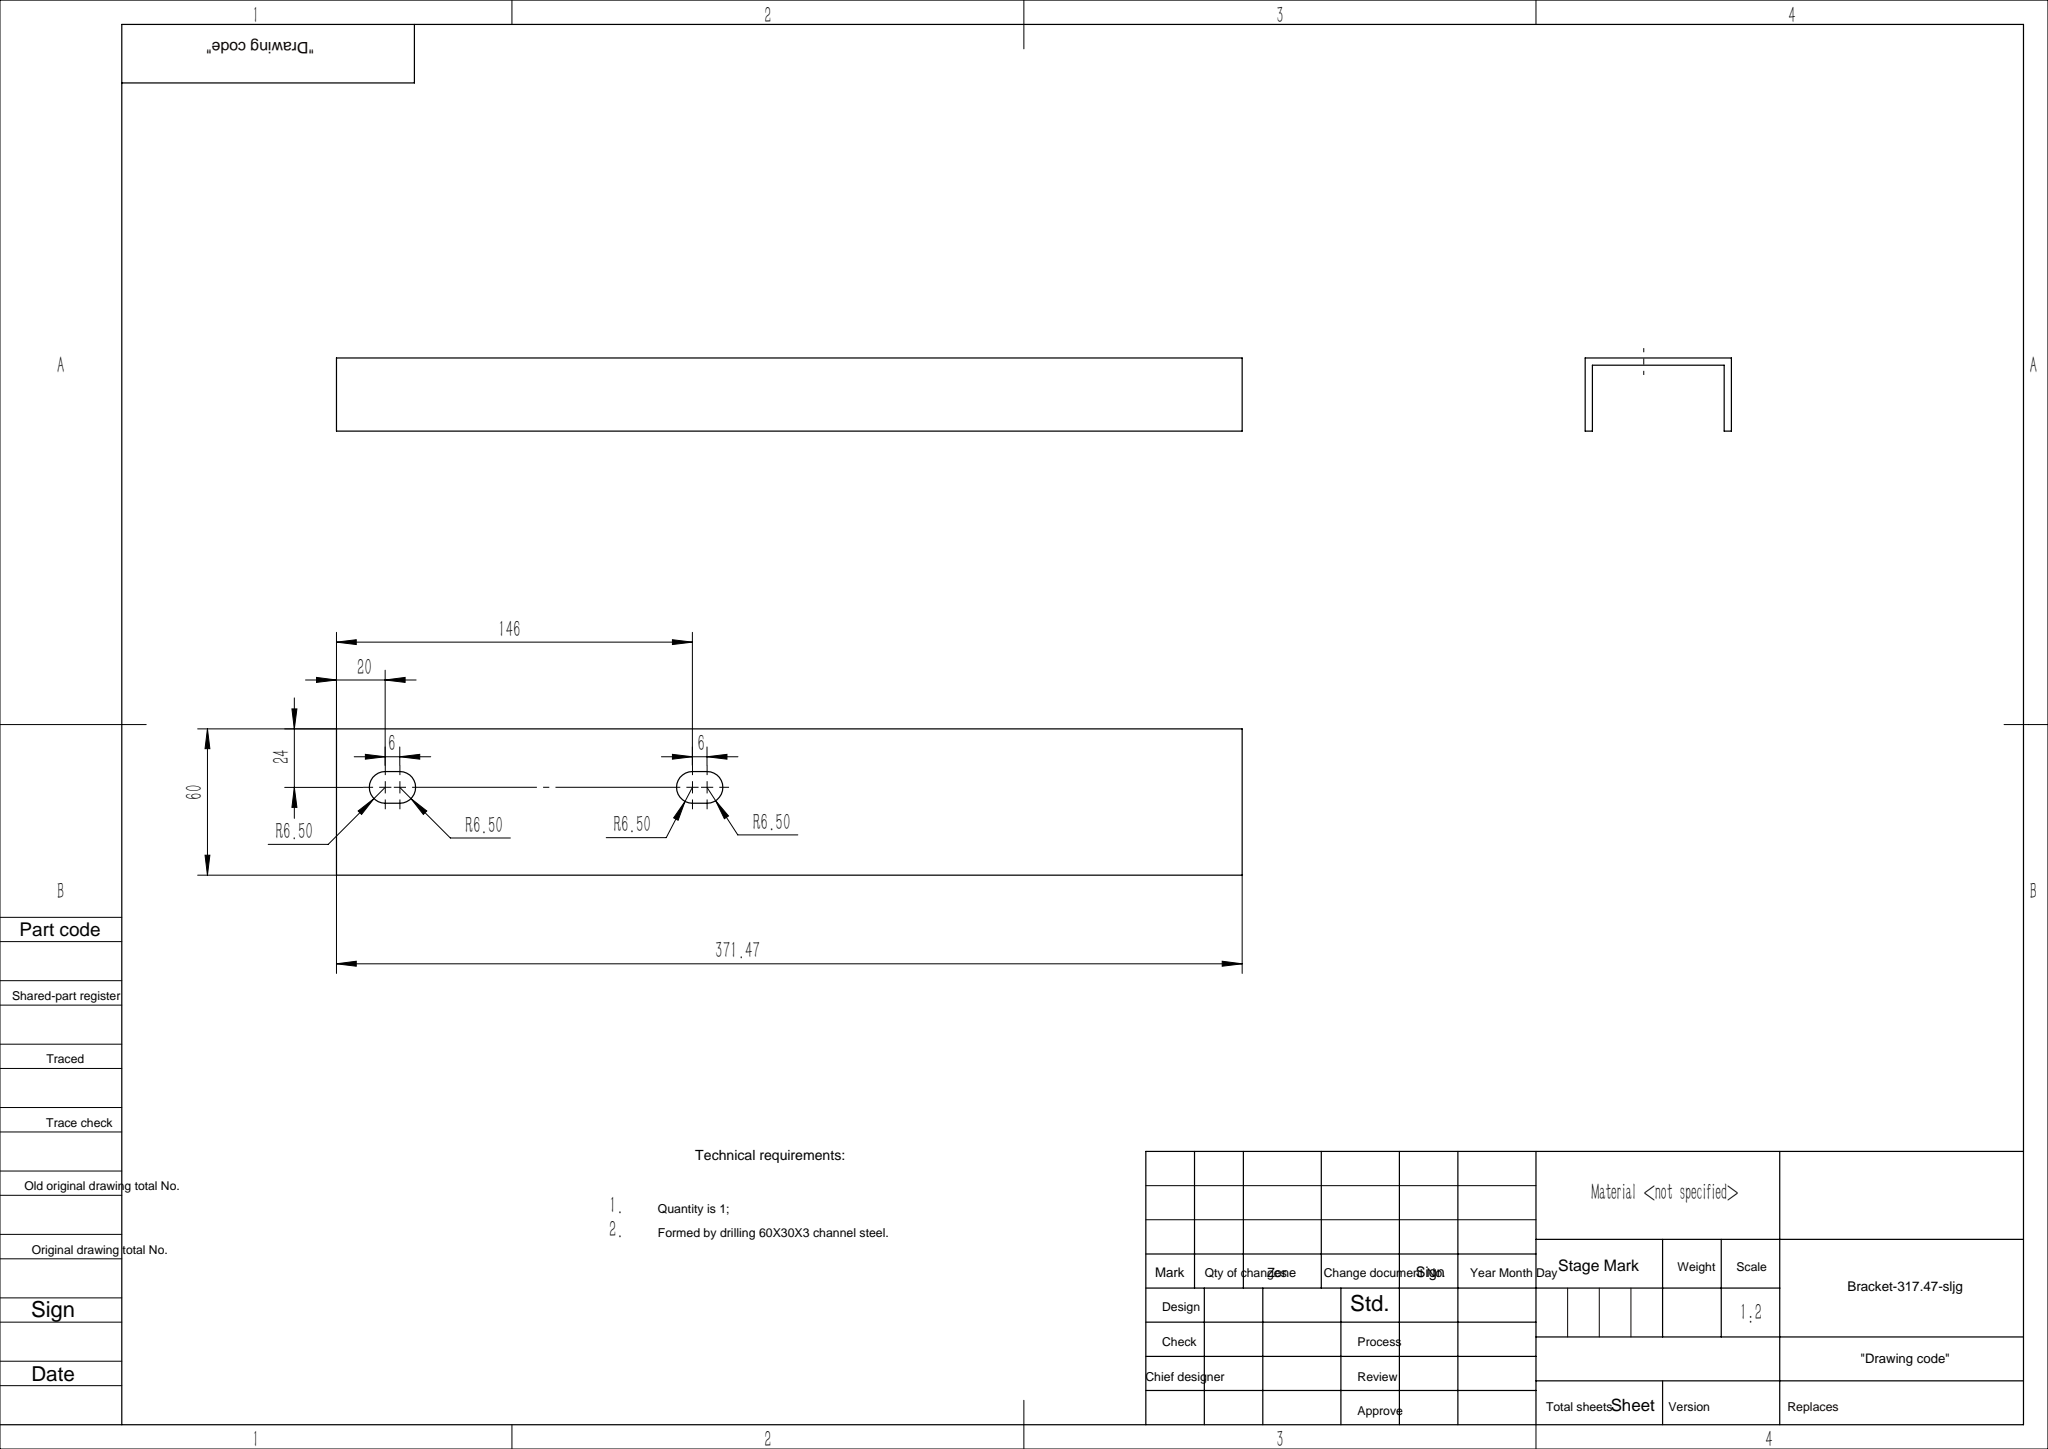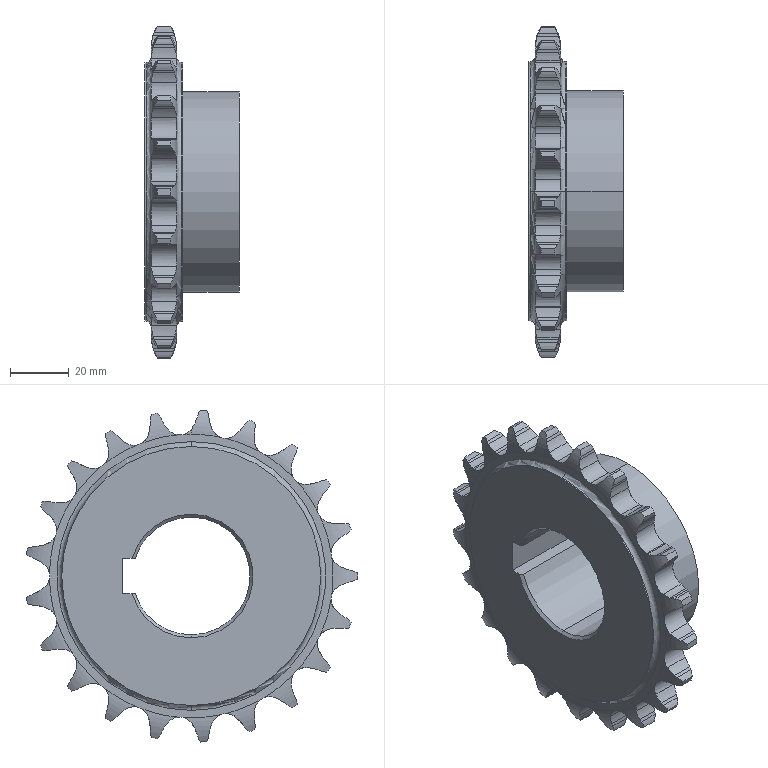Part | SolidWorks | features Chamfer 2, Cut 2, Revolution 2, CirPattern 1 | 1 solid | 249 faces | box 32 x 112.513 x 112.819 mm | volume 125263 mm3 | cylinder 145 | plane 50 | torus 48 | cone 6 | commonest cylinder face diameters 14.747 x44 26.567 x44 10.311 x27 113 x21 88 x4 40 x3